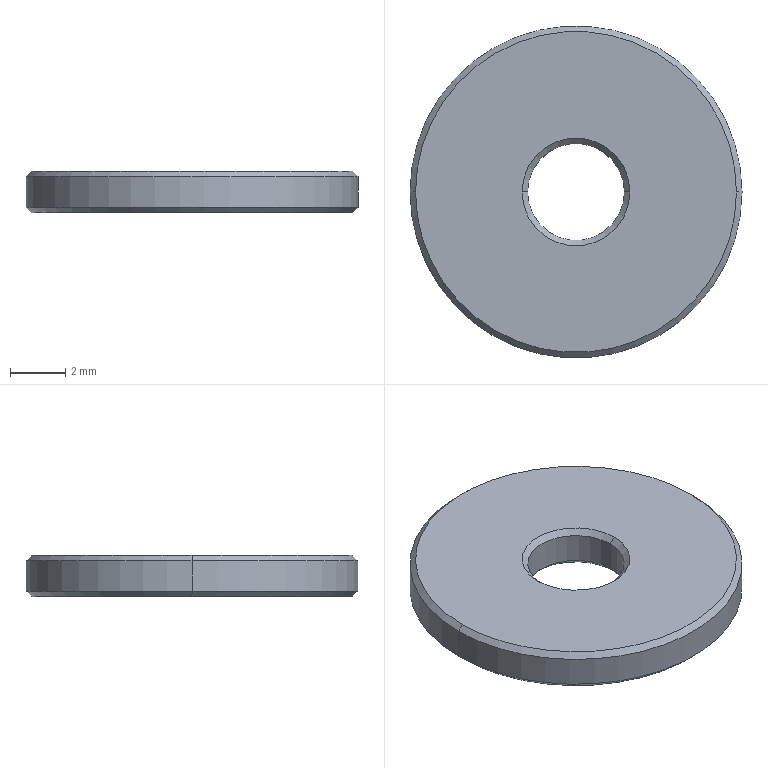Part | STEP file | 11-FG-SB00711 | 1 solid | 14 faces | box 12 x 12 x 1.5 mm | volume 153.267 mm3 | cone 8 | cylinder 4 | plane 2 | commonest cylinder face diameters 3.5 x2 12 x2
STEP:
#1=CARTESIAN_POINT('',(-1.75,0.,1.3));
#2=VERTEX_POINT('',#1);
#3=CARTESIAN_POINT('',(1.75,0.,1.3));
#4=VERTEX_POINT('',#3);
#5=CARTESIAN_POINT('',(0.,0.,1.3));
#6=DIRECTION('',(0.,0.,1.));
#7=DIRECTION('',(1.,0.,0.));
#8=AXIS2_PLACEMENT_3D('',#5,#6,#7);
#9=CIRCLE('',#8,1.75);
#10=EDGE_CURVE('',#2,#4,#9,.T.);
#11=ORIENTED_EDGE('',*,*,#10,.F.);
#12=CARTESIAN_POINT('',(-1.95,0.,1.5));
#13=VERTEX_POINT('',#12);
#14=CARTESIAN_POINT('',(-1.75,0.,1.3));
#15=DIRECTION('',(-0.7071,0.,0.7071));
#16=VECTOR('',#15,1000.);
#17=LINE('',#14,#16);
#18=EDGE_CURVE('',#2,#13,#17,.T.);
#19=ORIENTED_EDGE('',*,*,#18,.T.);
#20=CARTESIAN_POINT('',(1.95,0.,1.5));
#21=VERTEX_POINT('',#20);
#22=CARTESIAN_POINT('',(0.,0.,1.5));
#23=DIRECTION('',(0.,0.,-1.));
#24=DIRECTION('',(1.,0.,0.));
#25=AXIS2_PLACEMENT_3D('',#22,#23,#24);
#26=CIRCLE('',#25,1.95);
#27=EDGE_CURVE('',#21,#13,#26,.T.);
#28=ORIENTED_EDGE('',*,*,#27,.F.);
#29=CARTESIAN_POINT('',(1.75,0.,1.3));
#30=DIRECTION('',(0.7071,0.,0.7071));
#31=VECTOR('',#30,1000.);
#32=LINE('',#29,#31);
#33=EDGE_CURVE('',#4,#21,#32,.T.);
#34=ORIENTED_EDGE('',*,*,#33,.F.);
#35=EDGE_LOOP('',(#11,#19,#28,#34));
#36=FACE_OUTER_BOUND('',#35,.T.);
#37=CARTESIAN_POINT('',(0.,0.,1.3));
#38=DIRECTION('',(0.,0.,1.));
#39=DIRECTION('',(1.,0.,0.));
#40=AXIS2_PLACEMENT_3D('',#37,#38,#39);
#41=CONICAL_SURFACE('',#40,1.75,0.7854);
#42=ADVANCED_FACE('',(#36),#41,.F.);
#43=CARTESIAN_POINT('',(5.8,0.,1.5));
#44=VERTEX_POINT('',#43);
#45=CARTESIAN_POINT('',(-5.8,0.,1.5));
#46=VERTEX_POINT('',#45);
#47=CARTESIAN_POINT('',(0.,0.,1.5));
#48=DIRECTION('',(0.,0.,1.));
#49=DIRECTION('',(1.,0.,0.));
#50=AXIS2_PLACEMENT_3D('',#47,#48,#49);
#51=CIRCLE('',#50,5.8);
#52=EDGE_CURVE('',#44,#46,#51,.T.);
#53=ORIENTED_EDGE('',*,*,#52,.F.);
#54=CARTESIAN_POINT('',(6.,0.,1.3));
#55=VERTEX_POINT('',#54);
#56=CARTESIAN_POINT('',(5.8,0.,1.5));
#57=DIRECTION('',(0.7071,0.,-0.7071));
#58=VECTOR('',#57,1000.);
#59=LINE('',#56,#58);
#60=EDGE_CURVE('',#44,#55,#59,.T.);
#61=ORIENTED_EDGE('',*,*,#60,.T.);
#62=CARTESIAN_POINT('',(-6.,0.,1.3));
#63=VERTEX_POINT('',#62);
#64=CARTESIAN_POINT('',(0.,0.,1.3));
#65=DIRECTION('',(0.,0.,-1.));
#66=DIRECTION('',(1.,0.,0.));
#67=AXIS2_PLACEMENT_3D('',#64,#65,#66);
#68=CIRCLE('',#67,6.);
#69=EDGE_CURVE('',#63,#55,#68,.T.);
#70=ORIENTED_EDGE('',*,*,#69,.F.);
#71=CARTESIAN_POINT('',(-5.8,0.,1.5));
#72=DIRECTION('',(-0.7071,0.,-0.7071));
#73=VECTOR('',#72,1000.);
#74=LINE('',#71,#73);
#75=EDGE_CURVE('',#46,#63,#74,.T.);
#76=ORIENTED_EDGE('',*,*,#75,.F.);
#77=EDGE_LOOP('',(#53,#61,#70,#76));
#78=FACE_OUTER_BOUND('',#77,.T.);
#79=CARTESIAN_POINT('',(0.,0.,1.5));
#80=DIRECTION('',(0.,0.,-1.));
#81=DIRECTION('',(-1.,0.,0.));
#82=AXIS2_PLACEMENT_3D('',#79,#80,#81);
#83=CONICAL_SURFACE('',#82,5.8,0.7854);
#84=ADVANCED_FACE('',(#78),#83,.T.);
#85=CARTESIAN_POINT('',(-5.8,0.,0.));
#86=VERTEX_POINT('',#85);
#87=CARTESIAN_POINT('',(5.8,0.,0.));
#88=VERTEX_POINT('',#87);
#89=CARTESIAN_POINT('',(0.,0.,0.));
#90=DIRECTION('',(0.,0.,-1.));
#91=DIRECTION('',(1.,0.,0.));
#92=AXIS2_PLACEMENT_3D('',#89,#90,#91);
#93=CIRCLE('',#92,5.8);
#94=EDGE_CURVE('',#86,#88,#93,.T.);
#95=ORIENTED_EDGE('',*,*,#94,.F.);
#96=CARTESIAN_POINT('',(-6.,0.,0.2));
#97=VERTEX_POINT('',#96);
#98=CARTESIAN_POINT('',(-6.,0.,0.2));
#99=DIRECTION('',(-0.7071,0.,0.7071));
#100=VECTOR('',#99,1000.);
#101=LINE('',#98,#100);
#102=EDGE_CURVE('',#86,#97,#101,.T.);
#103=ORIENTED_EDGE('',*,*,#102,.T.);
#104=CARTESIAN_POINT('',(6.,0.,0.2));
#105=VERTEX_POINT('',#104);
#106=CARTESIAN_POINT('',(0.,0.,0.2));
#107=DIRECTION('',(0.,0.,1.));
#108=DIRECTION('',(1.,0.,0.));
#109=AXIS2_PLACEMENT_3D('',#106,#107,#108);
#110=CIRCLE('',#109,6.);
#111=EDGE_CURVE('',#105,#97,#110,.T.);
#112=ORIENTED_EDGE('',*,*,#111,.F.);
#113=CARTESIAN_POINT('',(6.,0.,0.2));
#114=DIRECTION('',(0.7071,0.,0.7071));
#115=VECTOR('',#114,1000.);
#116=LINE('',#113,#115);
#117=EDGE_CURVE('',#88,#105,#116,.T.);
#118=ORIENTED_EDGE('',*,*,#117,.F.);
#119=EDGE_LOOP('',(#95,#103,#112,#118));
#120=FACE_OUTER_BOUND('',#119,.T.);
#121=CARTESIAN_POINT('',(0.,0.,0.2));
#122=DIRECTION('',(0.,0.,1.));
#123=DIRECTION('',(1.,0.,0.));
#124=AXIS2_PLACEMENT_3D('',#121,#122,#123);
#125=CONICAL_SURFACE('',#124,6.,0.7854);
#126=ADVANCED_FACE('',(#120),#125,.T.);
#127=CARTESIAN_POINT('',(1.75,0.,0.2));
#128=VERTEX_POINT('',#127);
#129=CARTESIAN_POINT('',(-1.75,0.,0.2));
#130=VERTEX_POINT('',#129);
#131=CARTESIAN_POINT('',(0.,0.,0.2));
#132=DIRECTION('',(0.,0.,-1.));
#133=DIRECTION('',(1.,0.,0.));
#134=AXIS2_PLACEMENT_3D('',#131,#132,#133);
#135=CIRCLE('',#134,1.75);
#136=EDGE_CURVE('',#128,#130,#135,.T.);
#137=ORIENTED_EDGE('',*,*,#136,.F.);
#138=CARTESIAN_POINT('',(1.95,0.,0.));
#139=VERTEX_POINT('',#138);
#140=CARTESIAN_POINT('',(1.95,0.,0.));
#141=DIRECTION('',(0.7071,0.,-0.7071));
#142=VECTOR('',#141,1000.);
#143=LINE('',#140,#142);
#144=EDGE_CURVE('',#128,#139,#143,.T.);
#145=ORIENTED_EDGE('',*,*,#144,.T.);
#146=CARTESIAN_POINT('',(-1.95,0.,0.));
#147=VERTEX_POINT('',#146);
#148=CARTESIAN_POINT('',(0.,0.,0.));
#149=DIRECTION('',(0.,0.,1.));
#150=DIRECTION('',(1.,0.,0.));
#151=AXIS2_PLACEMENT_3D('',#148,#149,#150);
#152=CIRCLE('',#151,1.95);
#153=EDGE_CURVE('',#147,#139,#152,.T.);
#154=ORIENTED_EDGE('',*,*,#153,.F.);
#155=CARTESIAN_POINT('',(-1.95,0.,0.));
#156=DIRECTION('',(-0.7071,0.,-0.7071));
#157=VECTOR('',#156,1000.);
#158=LINE('',#155,#157);
#159=EDGE_CURVE('',#130,#147,#158,.T.);
#160=ORIENTED_EDGE('',*,*,#159,.F.);
#161=EDGE_LOOP('',(#137,#145,#154,#160));
#162=FACE_OUTER_BOUND('',#161,.T.);
#163=CARTESIAN_POINT('',(0.,0.,0.));
#164=DIRECTION('',(0.,0.,-1.));
#165=DIRECTION('',(-1.,0.,0.));
#166=AXIS2_PLACEMENT_3D('',#163,#164,#165);
#167=CONICAL_SURFACE('',#166,1.95,0.7854);
#168=ADVANCED_FACE('',(#162),#167,.F.);
#169=ORIENTED_EDGE('',*,*,#10,.T.);
#170=CARTESIAN_POINT('',(1.75,0.,1.5));
#171=DIRECTION('',(0.,0.,-1.));
#172=VECTOR('',#171,1000.);
#173=LINE('',#170,#172);
#174=EDGE_CURVE('',#4,#128,#173,.T.);
#175=ORIENTED_EDGE('',*,*,#174,.T.);
#176=ORIENTED_EDGE('',*,*,#136,.T.);
#177=CARTESIAN_POINT('',(-1.75,0.,1.5));
#178=DIRECTION('',(0.,0.,-1.));
#179=VECTOR('',#178,1000.);
#180=LINE('',#177,#179);
#181=EDGE_CURVE('',#2,#130,#180,.T.);
#182=ORIENTED_EDGE('',*,*,#181,.F.);
#183=EDGE_LOOP('',(#169,#175,#176,#182));
#184=FACE_OUTER_BOUND('',#183,.T.);
#185=CARTESIAN_POINT('',(0.,0.,1.5));
#186=DIRECTION('',(0.,0.,-1.));
#187=DIRECTION('',(-1.,0.,0.));
#188=AXIS2_PLACEMENT_3D('',#185,#186,#187);
#189=CYLINDRICAL_SURFACE('',#188,1.75);
#190=ADVANCED_FACE('',(#184),#189,.F.);
#191=ORIENTED_EDGE('',*,*,#69,.T.);
#192=CARTESIAN_POINT('',(6.,0.,1.5));
#193=DIRECTION('',(0.,0.,-1.));
#194=VECTOR('',#193,1000.);
#195=LINE('',#192,#194);
#196=EDGE_CURVE('',#55,#105,#195,.T.);
#197=ORIENTED_EDGE('',*,*,#196,.T.);
#198=ORIENTED_EDGE('',*,*,#111,.T.);
#199=CARTESIAN_POINT('',(-6.,0.,1.5));
#200=DIRECTION('',(0.,0.,-1.));
#201=VECTOR('',#200,1000.);
#202=LINE('',#199,#201);
#203=EDGE_CURVE('',#63,#97,#202,.T.);
#204=ORIENTED_EDGE('',*,*,#203,.F.);
#205=EDGE_LOOP('',(#191,#197,#198,#204));
#206=FACE_OUTER_BOUND('',#205,.T.);
#207=CARTESIAN_POINT('',(0.,0.,1.5));
#208=DIRECTION('',(0.,0.,-1.));
#209=DIRECTION('',(-1.,0.,0.));
#210=AXIS2_PLACEMENT_3D('',#207,#208,#209);
#211=CYLINDRICAL_SURFACE('',#210,6.);
#212=ADVANCED_FACE('',(#206),#211,.T.);
#213=CARTESIAN_POINT('',(0.,0.,1.5));
#214=DIRECTION('',(0.,0.,1.));
#215=DIRECTION('',(1.,0.,0.));
#216=AXIS2_PLACEMENT_3D('',#213,#214,#215);
#217=CIRCLE('',#216,5.8);
#218=EDGE_CURVE('',#46,#44,#217,.T.);
#219=ORIENTED_EDGE('',*,*,#218,.T.);
#220=ORIENTED_EDGE('',*,*,#52,.T.);
#221=EDGE_LOOP('',(#219,#220));
#222=FACE_OUTER_BOUND('',#221,.T.);
#223=ORIENTED_EDGE('',*,*,#27,.T.);
#224=CARTESIAN_POINT('',(0.,0.,1.5));
#225=DIRECTION('',(0.,0.,-1.));
#226=DIRECTION('',(1.,0.,0.));
#227=AXIS2_PLACEMENT_3D('',#224,#225,#226);
#228=CIRCLE('',#227,1.95);
#229=EDGE_CURVE('',#13,#21,#228,.T.);
#230=ORIENTED_EDGE('',*,*,#229,.T.);
#231=EDGE_LOOP('',(#223,#230));
#232=FACE_BOUND('',#231,.T.);
#233=CARTESIAN_POINT('',(0.,0.,1.5));
#234=DIRECTION('',(0.,0.,1.));
#235=DIRECTION('',(1.,0.,0.));
#236=AXIS2_PLACEMENT_3D('',#233,#234,#235);
#237=PLANE('',#236);
#238=ADVANCED_FACE('',(#222,#232),#237,.T.);
#239=ORIENTED_EDGE('',*,*,#153,.T.);
#240=CARTESIAN_POINT('',(0.,0.,0.));
#241=DIRECTION('',(0.,0.,1.));
#242=DIRECTION('',(1.,0.,0.));
#243=AXIS2_PLACEMENT_3D('',#240,#241,#242);
#244=CIRCLE('',#243,1.95);
#245=EDGE_CURVE('',#139,#147,#244,.T.);
#246=ORIENTED_EDGE('',*,*,#245,.T.);
#247=EDGE_LOOP('',(#239,#246));
#248=FACE_BOUND('',#247,.T.);
#249=CARTESIAN_POINT('',(0.,0.,0.));
#250=DIRECTION('',(0.,0.,-1.));
#251=DIRECTION('',(1.,0.,0.));
#252=AXIS2_PLACEMENT_3D('',#249,#250,#251);
#253=CIRCLE('',#252,5.8);
#254=EDGE_CURVE('',#88,#86,#253,.T.);
#255=ORIENTED_EDGE('',*,*,#254,.T.);
#256=ORIENTED_EDGE('',*,*,#94,.T.);
#257=EDGE_LOOP('',(#255,#256));
#258=FACE_OUTER_BOUND('',#257,.T.);
#259=CARTESIAN_POINT('',(0.,0.,0.));
#260=DIRECTION('',(0.,0.,1.));
#261=DIRECTION('',(1.,0.,0.));
#262=AXIS2_PLACEMENT_3D('',#259,#260,#261);
#263=PLANE('',#262);
#264=ADVANCED_FACE('',(#248,#258),#263,.F.);
#265=ORIENTED_EDGE('',*,*,#196,.F.);
#266=CARTESIAN_POINT('',(0.,0.,1.3));
#267=DIRECTION('',(0.,0.,-1.));
#268=DIRECTION('',(1.,0.,0.));
#269=AXIS2_PLACEMENT_3D('',#266,#267,#268);
#270=CIRCLE('',#269,6.);
#271=EDGE_CURVE('',#55,#63,#270,.T.);
#272=ORIENTED_EDGE('',*,*,#271,.T.);
#273=ORIENTED_EDGE('',*,*,#203,.T.);
#274=CARTESIAN_POINT('',(0.,0.,0.2));
#275=DIRECTION('',(0.,0.,1.));
#276=DIRECTION('',(1.,0.,0.));
#277=AXIS2_PLACEMENT_3D('',#274,#275,#276);
#278=CIRCLE('',#277,6.);
#279=EDGE_CURVE('',#97,#105,#278,.T.);
#280=ORIENTED_EDGE('',*,*,#279,.T.);
#281=EDGE_LOOP('',(#265,#272,#273,#280));
#282=FACE_OUTER_BOUND('',#281,.T.);
#283=CARTESIAN_POINT('',(0.,0.,1.5));
#284=DIRECTION('',(0.,0.,-1.));
#285=DIRECTION('',(-1.,0.,0.));
#286=AXIS2_PLACEMENT_3D('',#283,#284,#285);
#287=CYLINDRICAL_SURFACE('',#286,6.);
#288=ADVANCED_FACE('',(#282),#287,.T.);
#289=ORIENTED_EDGE('',*,*,#174,.F.);
#290=CARTESIAN_POINT('',(0.,0.,1.3));
#291=DIRECTION('',(0.,0.,1.));
#292=DIRECTION('',(1.,0.,0.));
#293=AXIS2_PLACEMENT_3D('',#290,#291,#292);
#294=CIRCLE('',#293,1.75);
#295=EDGE_CURVE('',#4,#2,#294,.T.);
#296=ORIENTED_EDGE('',*,*,#295,.T.);
#297=ORIENTED_EDGE('',*,*,#181,.T.);
#298=CARTESIAN_POINT('',(0.,0.,0.2));
#299=DIRECTION('',(0.,0.,-1.));
#300=DIRECTION('',(1.,0.,0.));
#301=AXIS2_PLACEMENT_3D('',#298,#299,#300);
#302=CIRCLE('',#301,1.75);
#303=EDGE_CURVE('',#130,#128,#302,.T.);
#304=ORIENTED_EDGE('',*,*,#303,.T.);
#305=EDGE_LOOP('',(#289,#296,#297,#304));
#306=FACE_OUTER_BOUND('',#305,.T.);
#307=CARTESIAN_POINT('',(0.,0.,1.5));
#308=DIRECTION('',(0.,0.,-1.));
#309=DIRECTION('',(-1.,0.,0.));
#310=AXIS2_PLACEMENT_3D('',#307,#308,#309);
#311=CYLINDRICAL_SURFACE('',#310,1.75);
#312=ADVANCED_FACE('',(#306),#311,.F.);
#313=ORIENTED_EDGE('',*,*,#144,.F.);
#314=ORIENTED_EDGE('',*,*,#303,.F.);
#315=ORIENTED_EDGE('',*,*,#159,.T.);
#316=ORIENTED_EDGE('',*,*,#245,.F.);
#317=EDGE_LOOP('',(#313,#314,#315,#316));
#318=FACE_OUTER_BOUND('',#317,.T.);
#319=CARTESIAN_POINT('',(0.,0.,0.));
#320=DIRECTION('',(0.,0.,-1.));
#321=DIRECTION('',(-1.,0.,0.));
#322=AXIS2_PLACEMENT_3D('',#319,#320,#321);
#323=CONICAL_SURFACE('',#322,1.95,0.7854);
#324=ADVANCED_FACE('',(#318),#323,.F.);
#325=ORIENTED_EDGE('',*,*,#102,.F.);
#326=ORIENTED_EDGE('',*,*,#254,.F.);
#327=ORIENTED_EDGE('',*,*,#117,.T.);
#328=ORIENTED_EDGE('',*,*,#279,.F.);
#329=EDGE_LOOP('',(#325,#326,#327,#328));
#330=FACE_OUTER_BOUND('',#329,.T.);
#331=CARTESIAN_POINT('',(0.,0.,0.2));
#332=DIRECTION('',(0.,0.,1.));
#333=DIRECTION('',(1.,0.,0.));
#334=AXIS2_PLACEMENT_3D('',#331,#332,#333);
#335=CONICAL_SURFACE('',#334,6.,0.7854);
#336=ADVANCED_FACE('',(#330),#335,.T.);
#337=ORIENTED_EDGE('',*,*,#60,.F.);
#338=ORIENTED_EDGE('',*,*,#218,.F.);
#339=ORIENTED_EDGE('',*,*,#75,.T.);
#340=ORIENTED_EDGE('',*,*,#271,.F.);
#341=EDGE_LOOP('',(#337,#338,#339,#340));
#342=FACE_OUTER_BOUND('',#341,.T.);
#343=CARTESIAN_POINT('',(0.,0.,1.5));
#344=DIRECTION('',(0.,0.,-1.));
#345=DIRECTION('',(-1.,0.,0.));
#346=AXIS2_PLACEMENT_3D('',#343,#344,#345);
#347=CONICAL_SURFACE('',#346,5.8,0.7854);
#348=ADVANCED_FACE('',(#342),#347,.T.);
#349=ORIENTED_EDGE('',*,*,#18,.F.);
#350=ORIENTED_EDGE('',*,*,#295,.F.);
#351=ORIENTED_EDGE('',*,*,#33,.T.);
#352=ORIENTED_EDGE('',*,*,#229,.F.);
#353=EDGE_LOOP('',(#349,#350,#351,#352));
#354=FACE_OUTER_BOUND('',#353,.T.);
#355=CARTESIAN_POINT('',(0.,0.,1.3));
#356=DIRECTION('',(0.,0.,1.));
#357=DIRECTION('',(1.,0.,0.));
#358=AXIS2_PLACEMENT_3D('',#355,#356,#357);
#359=CONICAL_SURFACE('',#358,1.75,0.7854);
#360=ADVANCED_FACE('',(#354),#359,.F.);
#361=CLOSED_SHELL('',(#42,#84,#126,#168,#190,#212,#238,#264,#288,#312,#324,#336,#348,#360));
#362=MANIFOLD_SOLID_BREP('',#361);
#363=CARTESIAN_POINT('',(0.,0.,0.));
#364=DIRECTION('',(0.,0.,1.));
#365=DIRECTION('',(1.,0.,0.));
#366=AXIS2_PLACEMENT_3D('',#363,#364,#365);
#367=(LENGTH_UNIT()NAMED_UNIT(*)SI_UNIT(.MILLI.,.METRE.));
#368=UNCERTAINTY_MEASURE_WITH_UNIT(LENGTH_MEASURE(0.00001),#367,'','');
#369=(NAMED_UNIT(*)PLANE_ANGLE_UNIT()SI_UNIT($,.RADIAN.));
#370=(NAMED_UNIT(*)SI_UNIT($,.STERADIAN.)SOLID_ANGLE_UNIT());
#371=(GEOMETRIC_REPRESENTATION_CONTEXT(3)GLOBAL_UNCERTAINTY_ASSIGNED_CONTEXT((#368))GLOBAL_UNIT_ASSIGNED_CONTEXT((#367,#369,#370))REPRESENTATION_CONTEXT('',''));
#372=ADVANCED_BREP_SHAPE_REPRESENTATION('',(#362,#366),#371);